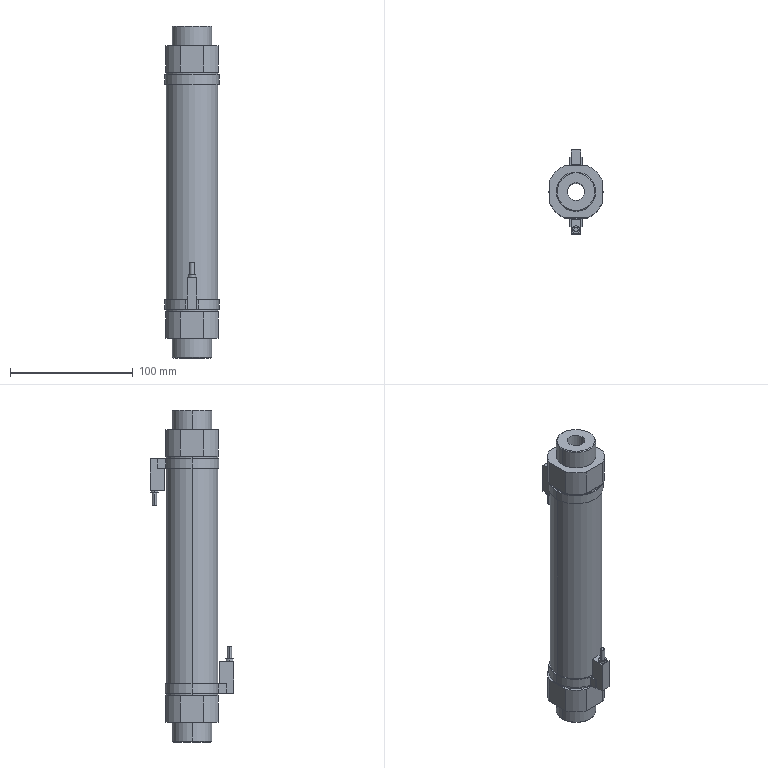Part | STEP file | body_A_CDM2WB40_150_C76_0_ | 1 solid | 95 faces | box 44 x 68 x 270 mm | volume 325918 mm3 | plane 47 | cylinder 40 | cone 8 | commonest cylinder face diameters 44 x8 46.5 x8 42 x6 3.4 x4 6 x4 11.45 x4